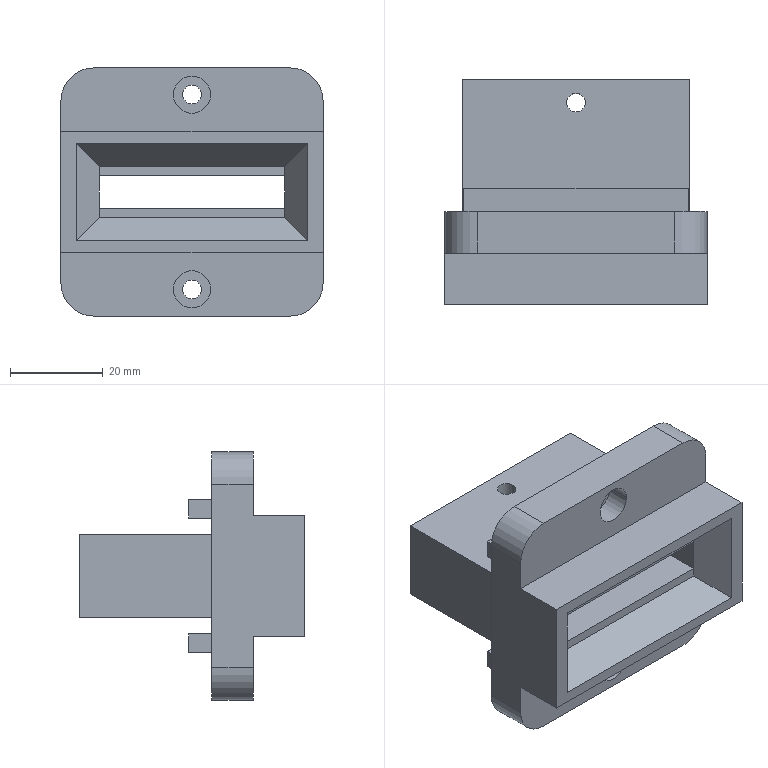Part | STEP file | BUSHING_INSULATOR_CXBY | 1 solid | 61 faces | box 56.5 x 48.5 x 53.5 mm | volume 51454 mm3 | plane 45 | cylinder 16 | commonest cylinder face diameters 4 x8 8 x4 14 x4